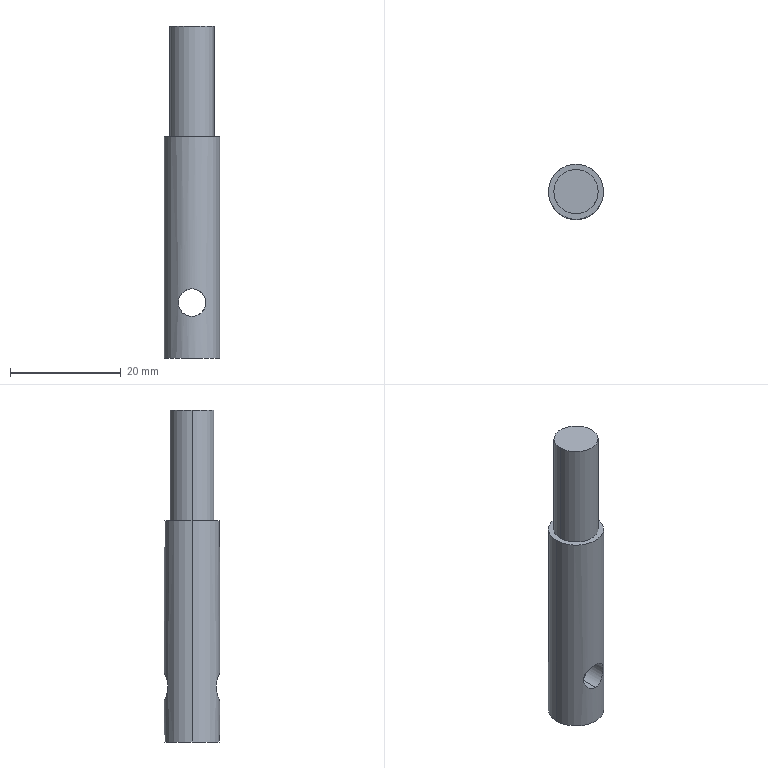Part | 1 solid | 11 faces | box 10 x 10 x 60 mm | volume 3892 mm3 | cylinder 8 | plane 3 | commonest cylinder face diameters 3.3 x2 5 x2 8 x2 10 x2
STEP:
#1=CARTESIAN_POINT('',(0.,-5.,7.5));
#2=VERTEX_POINT('',#1);
#3=CARTESIAN_POINT('',(0.,-5.,12.5));
#4=VERTEX_POINT('',#3);
#5=CARTESIAN_POINT('',(0.,-5.,7.5));
#6=CARTESIAN_POINT('',(-0.1657,-5.,7.5));
#7=CARTESIAN_POINT('',(-0.3343,-4.991,7.517));
#8=CARTESIAN_POINT('',(-0.6583,-4.959,7.583));
#9=CARTESIAN_POINT('',(-0.8154,-4.936,7.631));
#10=CARTESIAN_POINT('',(-1.12,-4.875,7.759));
#11=CARTESIAN_POINT('',(-1.263,-4.84,7.836));
#12=CARTESIAN_POINT('',(-1.531,-4.762,8.017));
#13=CARTESIAN_POINT('',(-1.657,-4.719,8.121));
#14=CARTESIAN_POINT('',(-1.884,-4.633,8.348));
#15=CARTESIAN_POINT('',(-1.985,-4.59,8.472));
#16=CARTESIAN_POINT('',(-2.165,-4.508,8.74));
#17=CARTESIAN_POINT('',(-2.243,-4.469,8.885));
#18=CARTESIAN_POINT('',(-2.368,-4.404,9.184));
#19=CARTESIAN_POINT('',(-2.417,-4.377,9.339));
#20=CARTESIAN_POINT('',(-2.483,-4.34,9.666));
#21=CARTESIAN_POINT('',(-2.5,-4.33,9.832));
#22=CARTESIAN_POINT('',(-2.5,-4.33,10.163));
#23=CARTESIAN_POINT('',(-2.484,-4.34,10.33));
#24=CARTESIAN_POINT('',(-2.418,-4.377,10.656));
#25=CARTESIAN_POINT('',(-2.37,-4.403,10.812));
#26=CARTESIAN_POINT('',(-2.181,-4.502,11.266));
#27=CARTESIAN_POINT('',(-1.997,-4.59,11.538));
#28=CARTESIAN_POINT('',(-1.655,-4.72,11.88));
#29=CARTESIAN_POINT('',(-1.532,-4.762,11.982));
#30=CARTESIAN_POINT('',(-1.264,-4.84,12.163));
#31=CARTESIAN_POINT('',(-1.119,-4.876,12.242));
#32=CARTESIAN_POINT('',(-0.8175,-4.935,12.368));
#33=CARTESIAN_POINT('',(-0.6613,-4.959,12.417));
#34=CARTESIAN_POINT('',(-0.3368,-4.991,12.483));
#35=CARTESIAN_POINT('',(-0.168,-5.,12.5));
#36=CARTESIAN_POINT('',(0.,-5.,12.5));
#37=B_SPLINE_CURVE_WITH_KNOTS('',3,(#5,#6,#7,#8,#9,#10,#11,#12,#13,#14,#15,#16,#17,#18,#19,#20,#21,#22,#23,#24,#25,#26,#27,#28,#29,#30,#31,#32,#33,#34,#35,#36),.UNSPECIFIED.,.F.,.F.,(4,2,2,2,2,2,2,2,2,2,2,2,2,2,2,4),(0.007952,0.008449,0.008945,0.009441,0.009937,0.01043,0.01093,0.01143,0.01192,0.01242,0.01291,0.01391,0.0144,0.0149,0.01539,0.01589),.UNSPECIFIED.);
#38=EDGE_CURVE('',#2,#4,#37,.T.);
#39=ORIENTED_EDGE('',*,*,#38,.F.);
#40=CARTESIAN_POINT('',(0.,-1.65,7.5));
#41=VERTEX_POINT('',#40);
#42=CARTESIAN_POINT('',(0.,-10.,7.5));
#43=DIRECTION('',(0.,1.,0.));
#44=VECTOR('',#43,1000.);
#45=LINE('',#42,#44);
#46=EDGE_CURVE('',#2,#41,#45,.T.);
#47=ORIENTED_EDGE('',*,*,#46,.T.);
#48=CARTESIAN_POINT('',(-1.65,0.,8.122));
#49=VERTEX_POINT('',#48);
#50=CARTESIAN_POINT('',(-1.65,0.,8.122));
#51=CARTESIAN_POINT('',(-1.65,-0.1131,8.122));
#52=CARTESIAN_POINT('',(-1.639,-0.2233,8.112));
#53=CARTESIAN_POINT('',(-1.594,-0.4385,8.074));
#54=CARTESIAN_POINT('',(-1.561,-0.5441,8.047));
#55=CARTESIAN_POINT('',(-1.436,-0.8398,7.951));
#56=CARTESIAN_POINT('',(-1.317,-1.016,7.868));
#57=CARTESIAN_POINT('',(-1.095,-1.238,7.751));
#58=CARTESIAN_POINT('',(-1.013,-1.307,7.713));
#59=CARTESIAN_POINT('',(-0.838,-1.425,7.643));
#60=CARTESIAN_POINT('',(-0.7448,-1.476,7.611));
#61=CARTESIAN_POINT('',(-0.5456,-1.561,7.558));
#62=CARTESIAN_POINT('',(-0.4386,-1.594,7.536));
#63=CARTESIAN_POINT('',(-0.2228,-1.639,7.508));
#64=CARTESIAN_POINT('',(-0.1126,-1.65,7.5));
#65=CARTESIAN_POINT('',(0.,-1.65,7.5));
#66=B_SPLINE_CURVE_WITH_KNOTS('',3,(#50,#51,#52,#53,#54,#55,#56,#57,#58,#59,#60,#61,#62,#63,#64,#65),.UNSPECIFIED.,.F.,.F.,(4,2,2,2,2,2,2,4),(0.,0.0003333,0.0006667,0.001333,0.001667,0.002,0.002333,0.002667),.UNSPECIFIED.);
#67=EDGE_CURVE('',#49,#41,#66,.T.);
#68=ORIENTED_EDGE('',*,*,#67,.F.);
#69=CARTESIAN_POINT('',(0.,1.65,7.5));
#70=VERTEX_POINT('',#69);
#71=CARTESIAN_POINT('',(0.,1.65,7.5));
#72=CARTESIAN_POINT('',(-0.1109,1.65,7.5));
#73=CARTESIAN_POINT('',(-0.2234,1.639,7.508));
#74=CARTESIAN_POINT('',(-0.4405,1.594,7.537));
#75=CARTESIAN_POINT('',(-0.5448,1.561,7.558));
#76=CARTESIAN_POINT('',(-0.8459,1.433,7.638));
#77=CARTESIAN_POINT('',(-1.023,1.311,7.713));
#78=CARTESIAN_POINT('',(-1.244,1.089,7.83));
#79=CARTESIAN_POINT('',(-1.31,1.009,7.87));
#80=CARTESIAN_POINT('',(-1.427,0.8346,7.946));
#81=CARTESIAN_POINT('',(-1.478,0.7407,7.983));
#82=CARTESIAN_POINT('',(-1.603,0.4463,8.078));
#83=CARTESIAN_POINT('',(-1.65,0.2251,8.122));
#84=CARTESIAN_POINT('',(-1.65,0.,8.122));
#85=B_SPLINE_CURVE_WITH_KNOTS('',3,(#71,#72,#73,#74,#75,#76,#77,#78,#79,#80,#81,#82,#83,#84),.UNSPECIFIED.,.F.,.F.,(4,2,2,2,2,2,4),(0.007982,0.008313,0.008645,0.009308,0.009639,0.009971,0.01063),.UNSPECIFIED.);
#86=EDGE_CURVE('',#70,#49,#85,.T.);
#87=ORIENTED_EDGE('',*,*,#86,.F.);
#88=CARTESIAN_POINT('',(0.,5.,7.5));
#89=VERTEX_POINT('',#88);
#90=CARTESIAN_POINT('',(0.,-10.,7.5));
#91=DIRECTION('',(0.,1.,0.));
#92=VECTOR('',#91,1000.);
#93=LINE('',#90,#92);
#94=EDGE_CURVE('',#70,#89,#93,.T.);
#95=ORIENTED_EDGE('',*,*,#94,.T.);
#96=CARTESIAN_POINT('',(0.,5.,12.5));
#97=VERTEX_POINT('',#96);
#98=CARTESIAN_POINT('',(0.,5.,12.5));
#99=CARTESIAN_POINT('',(-0.1682,5.,12.5));
#100=CARTESIAN_POINT('',(-0.3332,4.992,12.483));
#101=CARTESIAN_POINT('',(-0.6568,4.959,12.418));
#102=CARTESIAN_POINT('',(-0.8171,4.935,12.368));
#103=CARTESIAN_POINT('',(-1.27,4.846,12.178));
#104=CARTESIAN_POINT('',(-1.543,4.762,11.993));
#105=CARTESIAN_POINT('',(-1.883,4.633,11.652));
#106=CARTESIAN_POINT('',(-1.986,4.59,11.527));
#107=CARTESIAN_POINT('',(-2.166,4.507,11.258));
#108=CARTESIAN_POINT('',(-2.243,4.469,11.116));
#109=CARTESIAN_POINT('',(-2.368,4.404,10.817));
#110=CARTESIAN_POINT('',(-2.418,4.377,10.657));
#111=CARTESIAN_POINT('',(-2.483,4.34,10.333));
#112=CARTESIAN_POINT('',(-2.5,4.33,10.169));
#113=CARTESIAN_POINT('',(-2.5,4.33,9.836));
#114=CARTESIAN_POINT('',(-2.483,4.34,9.667));
#115=CARTESIAN_POINT('',(-2.418,4.377,9.344));
#116=CARTESIAN_POINT('',(-2.369,4.404,9.185));
#117=CARTESIAN_POINT('',(-2.242,4.47,8.883));
#118=CARTESIAN_POINT('',(-2.165,4.508,8.74));
#119=CARTESIAN_POINT('',(-1.985,4.59,8.472));
#120=CARTESIAN_POINT('',(-1.881,4.634,8.346));
#121=CARTESIAN_POINT('',(-1.541,4.763,8.006));
#122=CARTESIAN_POINT('',(-1.266,4.847,7.82));
#123=CARTESIAN_POINT('',(-0.8162,4.935,7.631));
#124=CARTESIAN_POINT('',(-0.6575,4.959,7.582));
#125=CARTESIAN_POINT('',(-0.3307,4.992,7.516));
#126=CARTESIAN_POINT('',(-0.166,5.,7.5));
#127=CARTESIAN_POINT('',(0.,5.,7.5));
#128=B_SPLINE_CURVE_WITH_KNOTS('',3,(#98,#99,#100,#101,#102,#103,#104,#105,#106,#107,#108,#109,#110,#111,#112,#113,#114,#115,#116,#117,#118,#119,#120,#121,#122,#123,#124,#125,#126,#127),.UNSPECIFIED.,.F.,.F.,(4,2,2,2,2,2,2,2,2,2,2,2,2,2,4),(0.,0.000497,0.0009941,0.001988,0.002485,0.002982,0.003479,0.003976,0.004473,0.00497,0.005467,0.005964,0.006958,0.007455,0.007952),.UNSPECIFIED.);
#129=EDGE_CURVE('',#97,#89,#128,.T.);
#130=ORIENTED_EDGE('',*,*,#129,.F.);
#131=CARTESIAN_POINT('',(0.,-10.,12.5));
#132=DIRECTION('',(0.,1.,0.));
#133=VECTOR('',#132,1000.);
#134=LINE('',#131,#133);
#135=EDGE_CURVE('',#4,#97,#134,.T.);
#136=ORIENTED_EDGE('',*,*,#135,.F.);
#137=EDGE_LOOP('',(#39,#47,#68,#87,#95,#130,#136));
#138=FACE_OUTER_BOUND('',#137,.T.);
#139=CARTESIAN_POINT('',(0.,-10.,10.));
#140=DIRECTION('',(0.,1.,0.));
#141=DIRECTION('',(0.,0.,1.));
#142=AXIS2_PLACEMENT_3D('',#139,#140,#141);
#143=CYLINDRICAL_SURFACE('',#142,2.5);
#144=ADVANCED_FACE('',(#138),#143,.F.);
#145=ORIENTED_EDGE('',*,*,#67,.T.);
#146=CARTESIAN_POINT('',(1.65,0.,8.122));
#147=VERTEX_POINT('',#146);
#148=CARTESIAN_POINT('',(0.,-1.65,7.5));
#149=CARTESIAN_POINT('',(0.2245,-1.65,7.5));
#150=CARTESIAN_POINT('',(0.4467,-1.603,7.532));
#151=CARTESIAN_POINT('',(0.8454,-1.433,7.638));
#152=CARTESIAN_POINT('',(1.023,-1.311,7.713));
#153=CARTESIAN_POINT('',(1.244,-1.089,7.83));
#154=CARTESIAN_POINT('',(1.311,-1.007,7.87));
#155=CARTESIAN_POINT('',(1.428,-0.8336,7.947));
#156=CARTESIAN_POINT('',(1.478,-0.7415,7.983));
#157=CARTESIAN_POINT('',(1.603,-0.4467,8.078));
#158=CARTESIAN_POINT('',(1.65,-0.2237,8.122));
#159=CARTESIAN_POINT('',(1.65,0.,8.122));
#160=B_SPLINE_CURVE_WITH_KNOTS('',3,(#148,#149,#150,#151,#152,#153,#154,#155,#156,#157,#158,#159),.UNSPECIFIED.,.F.,.F.,(4,2,2,2,2,4),(0.002667,0.003331,0.003996,0.004328,0.00466,0.005325),.UNSPECIFIED.);
#161=EDGE_CURVE('',#41,#147,#160,.T.);
#162=ORIENTED_EDGE('',*,*,#161,.T.);
#163=CARTESIAN_POINT('',(1.65,0.,0.));
#164=VERTEX_POINT('',#163);
#165=CARTESIAN_POINT('',(1.65,0.,0.));
#166=DIRECTION('',(0.,0.,-1.));
#167=VECTOR('',#166,1000.);
#168=LINE('',#165,#167);
#169=EDGE_CURVE('',#147,#164,#168,.T.);
#170=ORIENTED_EDGE('',*,*,#169,.T.);
#171=CARTESIAN_POINT('',(-1.65,0.,0.));
#172=VERTEX_POINT('',#171);
#173=CARTESIAN_POINT('',(0.,0.,0.));
#174=DIRECTION('',(0.,0.,-1.));
#175=DIRECTION('',(-1.,0.,0.));
#176=AXIS2_PLACEMENT_3D('',#173,#174,#175);
#177=CIRCLE('',#176,1.65);
#178=EDGE_CURVE('',#164,#172,#177,.T.);
#179=ORIENTED_EDGE('',*,*,#178,.T.);
#180=CARTESIAN_POINT('',(-1.65,0.,0.));
#181=DIRECTION('',(0.,0.,-1.));
#182=VECTOR('',#181,1000.);
#183=LINE('',#180,#182);
#184=EDGE_CURVE('',#49,#172,#183,.T.);
#185=ORIENTED_EDGE('',*,*,#184,.F.);
#186=EDGE_LOOP('',(#145,#162,#170,#179,#185));
#187=FACE_OUTER_BOUND('',#186,.T.);
#188=CARTESIAN_POINT('',(0.,0.,0.));
#189=DIRECTION('',(0.,0.,-1.));
#190=DIRECTION('',(-1.,0.,0.));
#191=AXIS2_PLACEMENT_3D('',#188,#189,#190);
#192=CYLINDRICAL_SURFACE('',#191,1.65);
#193=ADVANCED_FACE('',(#187),#192,.F.);
#194=CARTESIAN_POINT('',(4.,0.,60.));
#195=VERTEX_POINT('',#194);
#196=CARTESIAN_POINT('',(-4.,0.,60.));
#197=VERTEX_POINT('',#196);
#198=CARTESIAN_POINT('',(0.,0.,60.));
#199=DIRECTION('',(0.,0.,1.));
#200=DIRECTION('',(1.,0.,0.));
#201=AXIS2_PLACEMENT_3D('',#198,#199,#200);
#202=CIRCLE('',#201,4.);
#203=EDGE_CURVE('',#195,#197,#202,.T.);
#204=ORIENTED_EDGE('',*,*,#203,.F.);
#205=CARTESIAN_POINT('',(4.,0.,40.));
#206=VERTEX_POINT('',#205);
#207=CARTESIAN_POINT('',(4.,0.,60.));
#208=DIRECTION('',(0.,0.,-1.));
#209=VECTOR('',#208,1000.);
#210=LINE('',#207,#209);
#211=EDGE_CURVE('',#195,#206,#210,.T.);
#212=ORIENTED_EDGE('',*,*,#211,.T.);
#213=CARTESIAN_POINT('',(-4.,0.,40.));
#214=VERTEX_POINT('',#213);
#215=CARTESIAN_POINT('',(0.,0.,40.));
#216=DIRECTION('',(0.,0.,1.));
#217=DIRECTION('',(1.,0.,0.));
#218=AXIS2_PLACEMENT_3D('',#215,#216,#217);
#219=CIRCLE('',#218,4.);
#220=EDGE_CURVE('',#206,#214,#219,.T.);
#221=ORIENTED_EDGE('',*,*,#220,.T.);
#222=CARTESIAN_POINT('',(-4.,0.,60.));
#223=DIRECTION('',(0.,0.,-1.));
#224=VECTOR('',#223,1000.);
#225=LINE('',#222,#224);
#226=EDGE_CURVE('',#197,#214,#225,.T.);
#227=ORIENTED_EDGE('',*,*,#226,.F.);
#228=EDGE_LOOP('',(#204,#212,#221,#227));
#229=FACE_OUTER_BOUND('',#228,.T.);
#230=CARTESIAN_POINT('',(0.,0.,60.));
#231=DIRECTION('',(0.,0.,-1.));
#232=DIRECTION('',(-1.,0.,0.));
#233=AXIS2_PLACEMENT_3D('',#230,#231,#232);
#234=CYLINDRICAL_SURFACE('',#233,4.);
#235=ADVANCED_FACE('',(#229),#234,.T.);
#236=ORIENTED_EDGE('',*,*,#129,.T.);
#237=CARTESIAN_POINT('',(0.,5.,7.5));
#238=CARTESIAN_POINT('',(0.1657,5.,7.5));
#239=CARTESIAN_POINT('',(0.3343,4.991,7.517));
#240=CARTESIAN_POINT('',(0.6583,4.959,7.583));
#241=CARTESIAN_POINT('',(0.8154,4.936,7.631));
#242=CARTESIAN_POINT('',(1.12,4.875,7.759));
#243=CARTESIAN_POINT('',(1.263,4.84,7.836));
#244=CARTESIAN_POINT('',(1.531,4.762,8.017));
#245=CARTESIAN_POINT('',(1.657,4.719,8.121));
#246=CARTESIAN_POINT('',(1.884,4.633,8.348));
#247=CARTESIAN_POINT('',(1.985,4.59,8.472));
#248=CARTESIAN_POINT('',(2.165,4.508,8.74));
#249=CARTESIAN_POINT('',(2.243,4.469,8.885));
#250=CARTESIAN_POINT('',(2.368,4.404,9.184));
#251=CARTESIAN_POINT('',(2.417,4.377,9.339));
#252=CARTESIAN_POINT('',(2.483,4.34,9.666));
#253=CARTESIAN_POINT('',(2.5,4.33,9.832));
#254=CARTESIAN_POINT('',(2.5,4.33,10.163));
#255=CARTESIAN_POINT('',(2.484,4.34,10.33));
#256=CARTESIAN_POINT('',(2.418,4.377,10.656));
#257=CARTESIAN_POINT('',(2.37,4.403,10.812));
#258=CARTESIAN_POINT('',(2.181,4.502,11.266));
#259=CARTESIAN_POINT('',(1.997,4.59,11.538));
#260=CARTESIAN_POINT('',(1.655,4.72,11.88));
#261=CARTESIAN_POINT('',(1.532,4.762,11.982));
#262=CARTESIAN_POINT('',(1.264,4.84,12.163));
#263=CARTESIAN_POINT('',(1.119,4.876,12.242));
#264=CARTESIAN_POINT('',(0.8175,4.935,12.368));
#265=CARTESIAN_POINT('',(0.6613,4.959,12.417));
#266=CARTESIAN_POINT('',(0.3368,4.991,12.483));
#267=CARTESIAN_POINT('',(0.168,5.,12.5));
#268=CARTESIAN_POINT('',(0.,5.,12.5));
#269=B_SPLINE_CURVE_WITH_KNOTS('',3,(#237,#238,#239,#240,#241,#242,#243,#244,#245,#246,#247,#248,#249,#250,#251,#252,#253,#254,#255,#256,#257,#258,#259,#260,#261,#262,#263,#264,#265,#266,#267,#268),.UNSPECIFIED.,.F.,.F.,(4,2,2,2,2,2,2,2,2,2,2,2,2,2,2,4),(0.007952,0.008449,0.008945,0.009441,0.009937,0.01043,0.01093,0.01143,0.01192,0.01242,0.01291,0.01391,0.0144,0.0149,0.01539,0.01589),.UNSPECIFIED.);
#270=EDGE_CURVE('',#89,#97,#269,.T.);
#271=ORIENTED_EDGE('',*,*,#270,.T.);
#272=EDGE_LOOP('',(#236,#271));
#273=FACE_BOUND('',#272,.T.);
#274=CARTESIAN_POINT('',(5.,0.,40.));
#275=VERTEX_POINT('',#274);
#276=CARTESIAN_POINT('',(-5.,0.,40.));
#277=VERTEX_POINT('',#276);
#278=CARTESIAN_POINT('',(0.,0.,40.));
#279=DIRECTION('',(0.,0.,1.));
#280=DIRECTION('',(1.,0.,0.));
#281=AXIS2_PLACEMENT_3D('',#278,#279,#280);
#282=CIRCLE('',#281,5.);
#283=EDGE_CURVE('',#275,#277,#282,.T.);
#284=ORIENTED_EDGE('',*,*,#283,.F.);
#285=CARTESIAN_POINT('',(5.,0.,0.));
#286=VERTEX_POINT('',#285);
#287=CARTESIAN_POINT('',(5.,0.,40.));
#288=DIRECTION('',(0.,0.,-1.));
#289=VECTOR('',#288,1000.);
#290=LINE('',#287,#289);
#291=EDGE_CURVE('',#275,#286,#290,.T.);
#292=ORIENTED_EDGE('',*,*,#291,.T.);
#293=CARTESIAN_POINT('',(-5.,0.,0.));
#294=VERTEX_POINT('',#293);
#295=CARTESIAN_POINT('',(0.,0.,0.));
#296=DIRECTION('',(0.,0.,1.));
#297=DIRECTION('',(1.,0.,0.));
#298=AXIS2_PLACEMENT_3D('',#295,#296,#297);
#299=CIRCLE('',#298,5.);
#300=EDGE_CURVE('',#286,#294,#299,.T.);
#301=ORIENTED_EDGE('',*,*,#300,.T.);
#302=CARTESIAN_POINT('',(-5.,0.,40.));
#303=DIRECTION('',(0.,0.,-1.));
#304=VECTOR('',#303,1000.);
#305=LINE('',#302,#304);
#306=EDGE_CURVE('',#277,#294,#305,.T.);
#307=ORIENTED_EDGE('',*,*,#306,.F.);
#308=EDGE_LOOP('',(#284,#292,#301,#307));
#309=FACE_OUTER_BOUND('',#308,.T.);
#310=CARTESIAN_POINT('',(0.,0.,40.));
#311=DIRECTION('',(0.,0.,-1.));
#312=DIRECTION('',(-1.,0.,0.));
#313=AXIS2_PLACEMENT_3D('',#310,#311,#312);
#314=CYLINDRICAL_SURFACE('',#313,5.);
#315=ADVANCED_FACE('',(#273,#309),#314,.T.);
#316=CARTESIAN_POINT('',(0.,0.,40.));
#317=DIRECTION('',(0.,0.,1.));
#318=DIRECTION('',(1.,0.,0.));
#319=AXIS2_PLACEMENT_3D('',#316,#317,#318);
#320=CIRCLE('',#319,5.);
#321=EDGE_CURVE('',#277,#275,#320,.T.);
#322=ORIENTED_EDGE('',*,*,#321,.T.);
#323=ORIENTED_EDGE('',*,*,#283,.T.);
#324=EDGE_LOOP('',(#322,#323));
#325=FACE_OUTER_BOUND('',#324,.T.);
#326=CARTESIAN_POINT('',(0.,0.,40.));
#327=DIRECTION('',(0.,0.,1.));
#328=DIRECTION('',(1.,0.,0.));
#329=AXIS2_PLACEMENT_3D('',#326,#327,#328);
#330=CIRCLE('',#329,4.);
#331=EDGE_CURVE('',#214,#206,#330,.T.);
#332=ORIENTED_EDGE('',*,*,#331,.F.);
#333=ORIENTED_EDGE('',*,*,#220,.F.);
#334=EDGE_LOOP('',(#332,#333));
#335=FACE_BOUND('',#334,.T.);
#336=CARTESIAN_POINT('',(0.,0.,40.));
#337=DIRECTION('',(0.,0.,1.));
#338=DIRECTION('',(1.,0.,0.));
#339=AXIS2_PLACEMENT_3D('',#336,#337,#338);
#340=PLANE('',#339);
#341=ADVANCED_FACE('',(#325,#335),#340,.T.);
#342=ORIENTED_EDGE('',*,*,#291,.F.);
#343=ORIENTED_EDGE('',*,*,#321,.F.);
#344=ORIENTED_EDGE('',*,*,#306,.T.);
#345=CARTESIAN_POINT('',(0.,0.,0.));
#346=DIRECTION('',(0.,0.,1.));
#347=DIRECTION('',(1.,0.,0.));
#348=AXIS2_PLACEMENT_3D('',#345,#346,#347);
#349=CIRCLE('',#348,5.);
#350=EDGE_CURVE('',#294,#286,#349,.T.);
#351=ORIENTED_EDGE('',*,*,#350,.T.);
#352=EDGE_LOOP('',(#342,#343,#344,#351));
#353=FACE_OUTER_BOUND('',#352,.T.);
#354=CARTESIAN_POINT('',(0.,-5.,12.5));
#355=CARTESIAN_POINT('',(0.1682,-5.,12.5));
#356=CARTESIAN_POINT('',(0.3332,-4.992,12.483));
#357=CARTESIAN_POINT('',(0.6568,-4.959,12.418));
#358=CARTESIAN_POINT('',(0.8171,-4.935,12.368));
#359=CARTESIAN_POINT('',(1.27,-4.846,12.178));
#360=CARTESIAN_POINT('',(1.543,-4.762,11.993));
#361=CARTESIAN_POINT('',(1.883,-4.633,11.652));
#362=CARTESIAN_POINT('',(1.986,-4.59,11.527));
#363=CARTESIAN_POINT('',(2.166,-4.507,11.258));
#364=CARTESIAN_POINT('',(2.243,-4.469,11.116));
#365=CARTESIAN_POINT('',(2.368,-4.404,10.817));
#366=CARTESIAN_POINT('',(2.418,-4.377,10.657));
#367=CARTESIAN_POINT('',(2.483,-4.34,10.333));
#368=CARTESIAN_POINT('',(2.5,-4.33,10.169));
#369=CARTESIAN_POINT('',(2.5,-4.33,9.836));
#370=CARTESIAN_POINT('',(2.483,-4.34,9.667));
#371=CARTESIAN_POINT('',(2.418,-4.377,9.344));
#372=CARTESIAN_POINT('',(2.369,-4.404,9.185));
#373=CARTESIAN_POINT('',(2.242,-4.47,8.883));
#374=CARTESIAN_POINT('',(2.165,-4.508,8.74));
#375=CARTESIAN_POINT('',(1.985,-4.59,8.472));
#376=CARTESIAN_POINT('',(1.881,-4.634,8.346));
#377=CARTESIAN_POINT('',(1.541,-4.763,8.006));
#378=CARTESIAN_POINT('',(1.266,-4.847,7.82));
#379=CARTESIAN_POINT('',(0.8162,-4.935,7.631));
#380=CARTESIAN_POINT('',(0.6575,-4.959,7.582));
#381=CARTESIAN_POINT('',(0.3307,-4.992,7.516));
#382=CARTESIAN_POINT('',(0.166,-5.,7.5));
#383=CARTESIAN_POINT('',(0.,-5.,7.5));
#384=B_SPLINE_CURVE_WITH_KNOTS('',3,(#354,#355,#356,#357,#358,#359,#360,#361,#362,#363,#364,#365,#366,#367,#368,#369,#370,#371,#372,#373,#374,#375,#376,#377,#378,#379,#380,#381,#382,#383),.UNSPECIFIED.,.F.,.F.,(4,2,2,2,2,2,2,2,2,2,2,2,2,2,4),(0.,0.000497,0.0009941,0.001988,0.002485,0.002982,0.003479,0.003976,0.004473,0.00497,0.005467,0.005964,0.006958,0.007455,0.007952),.UNSPECIFIED.);
#385=EDGE_CURVE('',#4,#2,#384,.T.);
#386=ORIENTED_EDGE('',*,*,#385,.T.);
#387=ORIENTED_EDGE('',*,*,#38,.T.);
#388=EDGE_LOOP('',(#386,#387));
#389=FACE_BOUND('',#388,.T.);
#390=CARTESIAN_POINT('',(0.,0.,40.));
#391=DIRECTION('',(0.,0.,-1.));
#392=DIRECTION('',(-1.,0.,0.));
#393=AXIS2_PLACEMENT_3D('',#390,#391,#392);
#394=CYLINDRICAL_SURFACE('',#393,5.);
#395=ADVANCED_FACE('',(#353,#389),#394,.T.);
#396=CARTESIAN_POINT('',(0.,0.,0.));
#397=DIRECTION('',(0.,0.,-1.));
#398=DIRECTION('',(-1.,0.,0.));
#399=AXIS2_PLACEMENT_3D('',#396,#397,#398);
#400=CIRCLE('',#399,1.65);
#401=EDGE_CURVE('',#172,#164,#400,.T.);
#402=ORIENTED_EDGE('',*,*,#401,.F.);
#403=ORIENTED_EDGE('',*,*,#178,.F.);
#404=EDGE_LOOP('',(#402,#403));
#405=FACE_BOUND('',#404,.T.);
#406=ORIENTED_EDGE('',*,*,#350,.F.);
#407=ORIENTED_EDGE('',*,*,#300,.F.);
#408=EDGE_LOOP('',(#406,#407));
#409=FACE_OUTER_BOUND('',#408,.T.);
#410=CARTESIAN_POINT('',(0.,0.,0.));
#411=DIRECTION('',(0.,0.,1.));
#412=DIRECTION('',(1.,0.,0.));
#413=AXIS2_PLACEMENT_3D('',#410,#411,#412);
#414=PLANE('',#413);
#415=ADVANCED_FACE('',(#405,#409),#414,.F.);
#416=ORIENTED_EDGE('',*,*,#211,.F.);
#417=CARTESIAN_POINT('',(0.,0.,60.));
#418=DIRECTION('',(0.,0.,1.));
#419=DIRECTION('',(1.,0.,0.));
#420=AXIS2_PLACEMENT_3D('',#417,#418,#419);
#421=CIRCLE('',#420,4.);
#422=EDGE_CURVE('',#197,#195,#421,.T.);
#423=ORIENTED_EDGE('',*,*,#422,.F.);
#424=ORIENTED_EDGE('',*,*,#226,.T.);
#425=ORIENTED_EDGE('',*,*,#331,.T.);
#426=EDGE_LOOP('',(#416,#423,#424,#425));
#427=FACE_OUTER_BOUND('',#426,.T.);
#428=CARTESIAN_POINT('',(0.,0.,60.));
#429=DIRECTION('',(0.,0.,-1.));
#430=DIRECTION('',(-1.,0.,0.));
#431=AXIS2_PLACEMENT_3D('',#428,#429,#430);
#432=CYLINDRICAL_SURFACE('',#431,4.);
#433=ADVANCED_FACE('',(#427),#432,.T.);
#434=ORIENTED_EDGE('',*,*,#422,.T.);
#435=ORIENTED_EDGE('',*,*,#203,.T.);
#436=EDGE_LOOP('',(#434,#435));
#437=FACE_OUTER_BOUND('',#436,.T.);
#438=CARTESIAN_POINT('',(0.,0.,60.));
#439=DIRECTION('',(0.,0.,1.));
#440=DIRECTION('',(1.,0.,0.));
#441=AXIS2_PLACEMENT_3D('',#438,#439,#440);
#442=PLANE('',#441);
#443=ADVANCED_FACE('',(#437),#442,.T.);
#444=ORIENTED_EDGE('',*,*,#169,.F.);
#445=CARTESIAN_POINT('',(1.65,0.,8.122));
#446=CARTESIAN_POINT('',(1.65,0.2236,8.122));
#447=CARTESIAN_POINT('',(1.603,0.4445,8.079));
#448=CARTESIAN_POINT('',(1.437,0.8395,7.951));
#449=CARTESIAN_POINT('',(1.318,1.015,7.869));
#450=CARTESIAN_POINT('',(1.095,1.239,7.751));
#451=CARTESIAN_POINT('',(1.015,1.305,7.713));
#452=CARTESIAN_POINT('',(0.8404,1.424,7.644));
#453=CARTESIAN_POINT('',(0.7453,1.476,7.611));
#454=CARTESIAN_POINT('',(0.5453,1.561,7.558));
#455=CARTESIAN_POINT('',(0.4411,1.594,7.537));
#456=CARTESIAN_POINT('',(0.2234,1.639,7.508));
#457=CARTESIAN_POINT('',(0.1111,1.65,7.5));
#458=CARTESIAN_POINT('',(0.,1.65,7.5));
#459=B_SPLINE_CURVE_WITH_KNOTS('',3,(#445,#446,#447,#448,#449,#450,#451,#452,#453,#454,#455,#456,#457,#458),.UNSPECIFIED.,.F.,.F.,(4,2,2,2,2,2,4),(0.005325,0.005989,0.006653,0.006985,0.007317,0.007649,0.007982),.UNSPECIFIED.);
#460=EDGE_CURVE('',#147,#70,#459,.T.);
#461=ORIENTED_EDGE('',*,*,#460,.T.);
#462=ORIENTED_EDGE('',*,*,#86,.T.);
#463=ORIENTED_EDGE('',*,*,#184,.T.);
#464=ORIENTED_EDGE('',*,*,#401,.T.);
#465=EDGE_LOOP('',(#444,#461,#462,#463,#464));
#466=FACE_OUTER_BOUND('',#465,.T.);
#467=CARTESIAN_POINT('',(0.,0.,0.));
#468=DIRECTION('',(0.,0.,-1.));
#469=DIRECTION('',(-1.,0.,0.));
#470=AXIS2_PLACEMENT_3D('',#467,#468,#469);
#471=CYLINDRICAL_SURFACE('',#470,1.65);
#472=ADVANCED_FACE('',(#466),#471,.F.);
#473=ORIENTED_EDGE('',*,*,#46,.F.);
#474=ORIENTED_EDGE('',*,*,#385,.F.);
#475=ORIENTED_EDGE('',*,*,#135,.T.);
#476=ORIENTED_EDGE('',*,*,#270,.F.);
#477=ORIENTED_EDGE('',*,*,#94,.F.);
#478=ORIENTED_EDGE('',*,*,#460,.F.);
#479=ORIENTED_EDGE('',*,*,#161,.F.);
#480=EDGE_LOOP('',(#473,#474,#475,#476,#477,#478,#479));
#481=FACE_OUTER_BOUND('',#480,.T.);
#482=CARTESIAN_POINT('',(0.,-10.,10.));
#483=DIRECTION('',(0.,1.,0.));
#484=DIRECTION('',(0.,0.,1.));
#485=AXIS2_PLACEMENT_3D('',#482,#483,#484);
#486=CYLINDRICAL_SURFACE('',#485,2.5);
#487=ADVANCED_FACE('',(#481),#486,.F.);
#488=CLOSED_SHELL('',(#144,#193,#235,#315,#341,#395,#415,#433,#443,#472,#487));
#489=MANIFOLD_SOLID_BREP('',#488);
#490=CARTESIAN_POINT('',(0.,0.,0.));
#491=DIRECTION('',(0.,0.,1.));
#492=DIRECTION('',(1.,0.,0.));
#493=AXIS2_PLACEMENT_3D('',#490,#491,#492);
#494=(LENGTH_UNIT()NAMED_UNIT(*)SI_UNIT(.MILLI.,.METRE.));
#495=UNCERTAINTY_MEASURE_WITH_UNIT(LENGTH_MEASURE(0.00001),#494,'','');
#496=(NAMED_UNIT(*)PLANE_ANGLE_UNIT()SI_UNIT($,.RADIAN.));
#497=(NAMED_UNIT(*)SI_UNIT($,.STERADIAN.)SOLID_ANGLE_UNIT());
#498=(GEOMETRIC_REPRESENTATION_CONTEXT(3)GLOBAL_UNCERTAINTY_ASSIGNED_CONTEXT((#495))GLOBAL_UNIT_ASSIGNED_CONTEXT((#494,#496,#497))REPRESENTATION_CONTEXT('',''));
#499=ADVANCED_BREP_SHAPE_REPRESENTATION('',(#489,#493),#498);